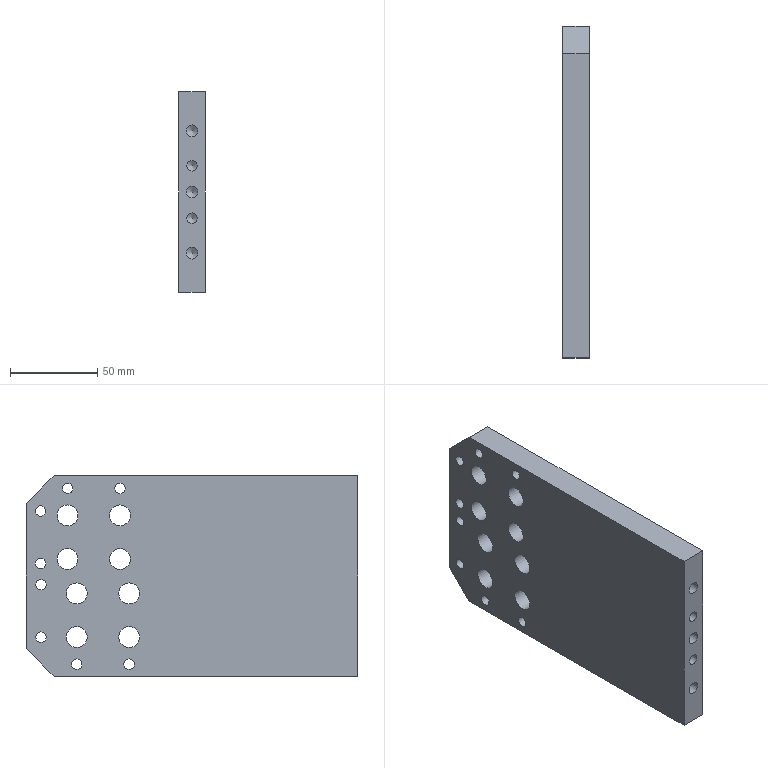Part | NX | features BREP 1 | 1 solid | 38 faces | box 15 x 190 x 115 mm | volume 303398 mm3 | cylinder 23 | plane 8 | cone 7 | commonest cylinder face diameters 6 x10 12 x8 6.8 x3 5 x2
STEP:
#1=CARTESIAN_POINT('',(-7.5,-95.,-57.5));
#2=VERTEX_POINT('',#1);
#3=CARTESIAN_POINT('',(-7.5,79.,-57.5));
#4=VERTEX_POINT('',#3);
#5=CARTESIAN_POINT('',(-7.5,-95.,-57.5));
#6=DIRECTION('',(0.,1.,0.));
#7=VECTOR('',#6,1000.);
#8=LINE('',#5,#7);
#9=EDGE_CURVE('',#2,#4,#8,.T.);
#10=ORIENTED_EDGE('',*,*,#9,.T.);
#11=CARTESIAN_POINT('',(7.5,79.,-57.5));
#12=VERTEX_POINT('',#11);
#13=CARTESIAN_POINT('',(7.5,79.,-57.5));
#14=DIRECTION('',(1.,0.,0.));
#15=VECTOR('',#14,1000.);
#16=LINE('',#13,#15);
#17=EDGE_CURVE('',#4,#12,#16,.T.);
#18=ORIENTED_EDGE('',*,*,#17,.T.);
#19=CARTESIAN_POINT('',(7.5,-95.,-57.5));
#20=VERTEX_POINT('',#19);
#21=CARTESIAN_POINT('',(7.5,-95.,-57.5));
#22=DIRECTION('',(0.,1.,0.));
#23=VECTOR('',#22,1000.);
#24=LINE('',#21,#23);
#25=EDGE_CURVE('',#20,#12,#24,.T.);
#26=ORIENTED_EDGE('',*,*,#25,.F.);
#27=CARTESIAN_POINT('',(7.5,-95.,-57.5));
#28=DIRECTION('',(-1.,0.,0.));
#29=VECTOR('',#28,1000.);
#30=LINE('',#27,#29);
#31=EDGE_CURVE('',#20,#2,#30,.T.);
#32=ORIENTED_EDGE('',*,*,#31,.T.);
#33=EDGE_LOOP('',(#10,#18,#26,#32));
#34=FACE_BOUND('',#33,.T.);
#35=CARTESIAN_POINT('',(7.5,-95.,-57.5));
#36=DIRECTION('',(0.,0.,1.));
#37=DIRECTION('',(-1.,0.,0.));
#38=AXIS2_PLACEMENT_3D('',#35,#36,#37);
#39=PLANE('',#38);
#40=ADVANCED_FACE('',(#34),#39,.F.);
#41=CARTESIAN_POINT('',(0.,95.,-14.5));
#42=VERTEX_POINT('',#41);
#43=CARTESIAN_POINT('',(0.,95.,-17.));
#44=DIRECTION('',(0.,1.,0.));
#45=DIRECTION('',(0.,0.,1.));
#46=AXIS2_PLACEMENT_3D('',#43,#44,#45);
#47=CIRCLE('',#46,2.5);
#48=EDGE_CURVE('',#42,#42,#47,.T.);
#49=ORIENTED_EDGE('',*,*,#48,.F.);
#50=EDGE_LOOP('',(#49));
#51=FACE_BOUND('',#50,.T.);
#52=CARTESIAN_POINT('',(0.,95.,25.5));
#53=VERTEX_POINT('',#52);
#54=CARTESIAN_POINT('',(0.,95.,23.));
#55=DIRECTION('',(0.,1.,0.));
#56=DIRECTION('',(0.,0.,1.));
#57=AXIS2_PLACEMENT_3D('',#54,#55,#56);
#58=CIRCLE('',#57,2.5);
#59=EDGE_CURVE('',#53,#53,#58,.T.);
#60=ORIENTED_EDGE('',*,*,#59,.F.);
#61=EDGE_LOOP('',(#60));
#62=FACE_BOUND('',#61,.T.);
#63=CARTESIAN_POINT('',(-7.5,95.,-41.5));
#64=VERTEX_POINT('',#63);
#65=CARTESIAN_POINT('',(-7.5,95.,41.5));
#66=VERTEX_POINT('',#65);
#67=CARTESIAN_POINT('',(-7.5,95.,57.5));
#68=DIRECTION('',(0.,0.,1.));
#69=VECTOR('',#68,1000.);
#70=LINE('',#67,#69);
#71=EDGE_CURVE('',#64,#66,#70,.T.);
#72=ORIENTED_EDGE('',*,*,#71,.T.);
#73=CARTESIAN_POINT('',(7.5,95.,41.5));
#74=VERTEX_POINT('',#73);
#75=CARTESIAN_POINT('',(7.5,95.,41.5));
#76=DIRECTION('',(1.,0.,0.));
#77=VECTOR('',#76,1000.);
#78=LINE('',#75,#77);
#79=EDGE_CURVE('',#66,#74,#78,.T.);
#80=ORIENTED_EDGE('',*,*,#79,.T.);
#81=CARTESIAN_POINT('',(7.5,95.,-41.5));
#82=VERTEX_POINT('',#81);
#83=CARTESIAN_POINT('',(7.5,95.,57.5));
#84=DIRECTION('',(0.,0.,1.));
#85=VECTOR('',#84,1000.);
#86=LINE('',#83,#85);
#87=EDGE_CURVE('',#82,#74,#86,.T.);
#88=ORIENTED_EDGE('',*,*,#87,.F.);
#89=CARTESIAN_POINT('',(7.5,95.,-41.5));
#90=DIRECTION('',(-1.,0.,0.));
#91=VECTOR('',#90,1000.);
#92=LINE('',#89,#91);
#93=EDGE_CURVE('',#82,#64,#92,.T.);
#94=ORIENTED_EDGE('',*,*,#93,.T.);
#95=EDGE_LOOP('',(#72,#80,#88,#94));
#96=FACE_BOUND('',#95,.T.);
#97=CARTESIAN_POINT('',(7.5,95.,57.5));
#98=DIRECTION('',(0.,-1.,0.));
#99=DIRECTION('',(0.,0.,1.));
#100=AXIS2_PLACEMENT_3D('',#97,#98,#99);
#101=PLANE('',#100);
#102=ADVANCED_FACE('',(#51,#62,#96),#101,.F.);
#103=CARTESIAN_POINT('',(7.5,79.,57.5));
#104=VERTEX_POINT('',#103);
#105=CARTESIAN_POINT('',(7.5,-95.,57.5));
#106=VERTEX_POINT('',#105);
#107=CARTESIAN_POINT('',(7.5,-95.,57.5));
#108=DIRECTION('',(0.,-1.,0.));
#109=VECTOR('',#108,1000.);
#110=LINE('',#107,#109);
#111=EDGE_CURVE('',#104,#106,#110,.T.);
#112=ORIENTED_EDGE('',*,*,#111,.F.);
#113=CARTESIAN_POINT('',(-7.5,79.,57.5));
#114=VERTEX_POINT('',#113);
#115=CARTESIAN_POINT('',(7.5,79.,57.5));
#116=DIRECTION('',(-1.,0.,0.));
#117=VECTOR('',#116,1000.);
#118=LINE('',#115,#117);
#119=EDGE_CURVE('',#104,#114,#118,.T.);
#120=ORIENTED_EDGE('',*,*,#119,.T.);
#121=CARTESIAN_POINT('',(-7.5,-95.,57.5));
#122=VERTEX_POINT('',#121);
#123=CARTESIAN_POINT('',(-7.5,-95.,57.5));
#124=DIRECTION('',(0.,-1.,0.));
#125=VECTOR('',#124,1000.);
#126=LINE('',#123,#125);
#127=EDGE_CURVE('',#114,#122,#126,.T.);
#128=ORIENTED_EDGE('',*,*,#127,.T.);
#129=CARTESIAN_POINT('',(7.5,-95.,57.5));
#130=DIRECTION('',(-1.,0.,0.));
#131=VECTOR('',#130,1000.);
#132=LINE('',#129,#131);
#133=EDGE_CURVE('',#106,#122,#132,.T.);
#134=ORIENTED_EDGE('',*,*,#133,.F.);
#135=EDGE_LOOP('',(#112,#120,#128,#134));
#136=FACE_BOUND('',#135,.T.);
#137=CARTESIAN_POINT('',(7.5,-95.,57.5));
#138=DIRECTION('',(0.,0.,-1.));
#139=DIRECTION('',(1.,0.,0.));
#140=AXIS2_PLACEMENT_3D('',#137,#138,#139);
#141=PLANE('',#140);
#142=ADVANCED_FACE('',(#136),#141,.F.);
#143=CARTESIAN_POINT('',(0.,-95.,-18.));
#144=VERTEX_POINT('',#143);
#145=CARTESIAN_POINT('',(0.,-95.,-15.));
#146=DIRECTION('',(0.,-1.,0.));
#147=DIRECTION('',(0.,0.,-1.));
#148=AXIS2_PLACEMENT_3D('',#145,#146,#147);
#149=CIRCLE('',#148,3.);
#150=EDGE_CURVE('',#144,#144,#149,.T.);
#151=ORIENTED_EDGE('',*,*,#150,.F.);
#152=EDGE_LOOP('',(#151));
#153=FACE_BOUND('',#152,.T.);
#154=CARTESIAN_POINT('',(0.,-95.,12.));
#155=VERTEX_POINT('',#154);
#156=CARTESIAN_POINT('',(0.,-95.,15.));
#157=DIRECTION('',(0.,-1.,0.));
#158=DIRECTION('',(0.,0.,-1.));
#159=AXIS2_PLACEMENT_3D('',#156,#157,#158);
#160=CIRCLE('',#159,3.);
#161=EDGE_CURVE('',#155,#155,#160,.T.);
#162=ORIENTED_EDGE('',*,*,#161,.F.);
#163=EDGE_LOOP('',(#162));
#164=FACE_BOUND('',#163,.T.);
#165=CARTESIAN_POINT('',(0.,-95.,31.6));
#166=VERTEX_POINT('',#165);
#167=CARTESIAN_POINT('',(0.,-95.,35.));
#168=DIRECTION('',(0.,-1.,0.));
#169=DIRECTION('',(0.,0.,-1.));
#170=AXIS2_PLACEMENT_3D('',#167,#168,#169);
#171=CIRCLE('',#170,3.4);
#172=EDGE_CURVE('',#166,#166,#171,.T.);
#173=ORIENTED_EDGE('',*,*,#172,.F.);
#174=EDGE_LOOP('',(#173));
#175=FACE_BOUND('',#174,.T.);
#176=CARTESIAN_POINT('',(0.,-95.,-38.4));
#177=VERTEX_POINT('',#176);
#178=CARTESIAN_POINT('',(0.,-95.,-35.));
#179=DIRECTION('',(0.,-1.,0.));
#180=DIRECTION('',(0.,0.,-1.));
#181=AXIS2_PLACEMENT_3D('',#178,#179,#180);
#182=CIRCLE('',#181,3.4);
#183=EDGE_CURVE('',#177,#177,#182,.T.);
#184=ORIENTED_EDGE('',*,*,#183,.F.);
#185=EDGE_LOOP('',(#184));
#186=FACE_BOUND('',#185,.T.);
#187=CARTESIAN_POINT('',(0.,-95.,-3.4));
#188=VERTEX_POINT('',#187);
#189=CARTESIAN_POINT('',(0.,-95.,0.));
#190=DIRECTION('',(0.,-1.,0.));
#191=DIRECTION('',(0.,0.,-1.));
#192=AXIS2_PLACEMENT_3D('',#189,#190,#191);
#193=CIRCLE('',#192,3.4);
#194=EDGE_CURVE('',#188,#188,#193,.T.);
#195=ORIENTED_EDGE('',*,*,#194,.F.);
#196=EDGE_LOOP('',(#195));
#197=FACE_BOUND('',#196,.T.);
#198=CARTESIAN_POINT('',(-7.5,-95.,57.5));
#199=DIRECTION('',(0.,0.,-1.));
#200=VECTOR('',#199,1000.);
#201=LINE('',#198,#200);
#202=EDGE_CURVE('',#122,#2,#201,.T.);
#203=ORIENTED_EDGE('',*,*,#202,.T.);
#204=ORIENTED_EDGE('',*,*,#31,.F.);
#205=CARTESIAN_POINT('',(7.5,-95.,57.5));
#206=DIRECTION('',(0.,0.,-1.));
#207=VECTOR('',#206,1000.);
#208=LINE('',#205,#207);
#209=EDGE_CURVE('',#106,#20,#208,.T.);
#210=ORIENTED_EDGE('',*,*,#209,.F.);
#211=ORIENTED_EDGE('',*,*,#133,.T.);
#212=EDGE_LOOP('',(#203,#204,#210,#211));
#213=FACE_BOUND('',#212,.T.);
#214=CARTESIAN_POINT('',(7.5,-95.,57.5));
#215=DIRECTION('',(0.,1.,0.));
#216=DIRECTION('',(0.,0.,-1.));
#217=AXIS2_PLACEMENT_3D('',#214,#215,#216);
#218=PLANE('',#217);
#219=ADVANCED_FACE('',(#153,#164,#175,#186,#197,#213),#218,.F.);
#220=CARTESIAN_POINT('',(7.5,66.,-53.5));
#221=VERTEX_POINT('',#220);
#222=CARTESIAN_POINT('',(7.5,66.,-50.5));
#223=DIRECTION('',(1.,0.,0.));
#224=DIRECTION('',(0.,0.,-1.));
#225=AXIS2_PLACEMENT_3D('',#222,#223,#224);
#226=CIRCLE('',#225,3.);
#227=EDGE_CURVE('',#221,#221,#226,.T.);
#228=ORIENTED_EDGE('',*,*,#227,.F.);
#229=EDGE_LOOP('',(#228));
#230=FACE_BOUND('',#229,.T.);
#231=CARTESIAN_POINT('',(7.5,36.,-53.5));
#232=VERTEX_POINT('',#231);
#233=CARTESIAN_POINT('',(7.5,36.,-50.5));
#234=DIRECTION('',(1.,0.,0.));
#235=DIRECTION('',(0.,0.,-1.));
#236=AXIS2_PLACEMENT_3D('',#233,#234,#235);
#237=CIRCLE('',#236,3.);
#238=EDGE_CURVE('',#232,#232,#237,.T.);
#239=ORIENTED_EDGE('',*,*,#238,.F.);
#240=EDGE_LOOP('',(#239));
#241=FACE_BOUND('',#240,.T.);
#242=CARTESIAN_POINT('',(7.5,86.5,-38.));
#243=VERTEX_POINT('',#242);
#244=CARTESIAN_POINT('',(7.5,86.5,-35.));
#245=DIRECTION('',(1.,0.,0.));
#246=DIRECTION('',(0.,0.,-1.));
#247=AXIS2_PLACEMENT_3D('',#244,#245,#246);
#248=CIRCLE('',#247,3.);
#249=EDGE_CURVE('',#243,#243,#248,.T.);
#250=ORIENTED_EDGE('',*,*,#249,.F.);
#251=EDGE_LOOP('',(#250));
#252=FACE_BOUND('',#251,.T.);
#253=CARTESIAN_POINT('',(7.5,86.5,-8.));
#254=VERTEX_POINT('',#253);
#255=CARTESIAN_POINT('',(7.5,86.5,-5.));
#256=DIRECTION('',(1.,0.,0.));
#257=DIRECTION('',(0.,0.,-1.));
#258=AXIS2_PLACEMENT_3D('',#255,#256,#257);
#259=CIRCLE('',#258,3.);
#260=EDGE_CURVE('',#254,#254,#259,.T.);
#261=ORIENTED_EDGE('',*,*,#260,.F.);
#262=EDGE_LOOP('',(#261));
#263=FACE_BOUND('',#262,.T.);
#264=CARTESIAN_POINT('',(7.5,86.759,4.207));
#265=VERTEX_POINT('',#264);
#266=CARTESIAN_POINT('',(7.5,86.759,7.207));
#267=DIRECTION('',(1.,0.,0.));
#268=DIRECTION('',(0.,0.,-1.));
#269=AXIS2_PLACEMENT_3D('',#266,#267,#268);
#270=CIRCLE('',#269,3.);
#271=EDGE_CURVE('',#265,#265,#270,.T.);
#272=ORIENTED_EDGE('',*,*,#271,.F.);
#273=EDGE_LOOP('',(#272));
#274=FACE_BOUND('',#273,.T.);
#275=CARTESIAN_POINT('',(7.5,86.759,34.207));
#276=VERTEX_POINT('',#275);
#277=CARTESIAN_POINT('',(7.5,86.759,37.207));
#278=DIRECTION('',(1.,0.,0.));
#279=DIRECTION('',(0.,0.,-1.));
#280=AXIS2_PLACEMENT_3D('',#277,#278,#279);
#281=CIRCLE('',#280,3.);
#282=EDGE_CURVE('',#276,#276,#281,.T.);
#283=ORIENTED_EDGE('',*,*,#282,.F.);
#284=EDGE_LOOP('',(#283));
#285=FACE_BOUND('',#284,.T.);
#286=CARTESIAN_POINT('',(7.5,71.259,47.207));
#287=VERTEX_POINT('',#286);
#288=CARTESIAN_POINT('',(7.5,71.259,50.207));
#289=DIRECTION('',(1.,0.,0.));
#290=DIRECTION('',(0.,0.,-1.));
#291=AXIS2_PLACEMENT_3D('',#288,#289,#290);
#292=CIRCLE('',#291,3.);
#293=EDGE_CURVE('',#287,#287,#292,.T.);
#294=ORIENTED_EDGE('',*,*,#293,.F.);
#295=EDGE_LOOP('',(#294));
#296=FACE_BOUND('',#295,.T.);
#297=CARTESIAN_POINT('',(7.5,41.259,47.207));
#298=VERTEX_POINT('',#297);
#299=CARTESIAN_POINT('',(7.5,41.259,50.207));
#300=DIRECTION('',(1.,0.,0.));
#301=DIRECTION('',(0.,0.,-1.));
#302=AXIS2_PLACEMENT_3D('',#299,#300,#301);
#303=CIRCLE('',#302,3.);
#304=EDGE_CURVE('',#298,#298,#303,.T.);
#305=ORIENTED_EDGE('',*,*,#304,.F.);
#306=EDGE_LOOP('',(#305));
#307=FACE_BOUND('',#306,.T.);
#308=CARTESIAN_POINT('',(7.5,36.,-29.));
#309=VERTEX_POINT('',#308);
#310=CARTESIAN_POINT('',(7.5,36.,-35.));
#311=DIRECTION('',(-1.,0.,0.));
#312=DIRECTION('',(0.,0.,1.));
#313=AXIS2_PLACEMENT_3D('',#310,#311,#312);
#314=CIRCLE('',#313,6.);
#315=EDGE_CURVE('',#309,#309,#314,.T.);
#316=ORIENTED_EDGE('',*,*,#315,.T.);
#317=EDGE_LOOP('',(#316));
#318=FACE_BOUND('',#317,.T.);
#319=CARTESIAN_POINT('',(7.5,36.,-4.));
#320=VERTEX_POINT('',#319);
#321=CARTESIAN_POINT('',(7.5,36.,-10.));
#322=DIRECTION('',(-1.,0.,0.));
#323=DIRECTION('',(0.,0.,1.));
#324=AXIS2_PLACEMENT_3D('',#321,#322,#323);
#325=CIRCLE('',#324,6.);
#326=EDGE_CURVE('',#320,#320,#325,.T.);
#327=ORIENTED_EDGE('',*,*,#326,.T.);
#328=EDGE_LOOP('',(#327));
#329=FACE_BOUND('',#328,.T.);
#330=CARTESIAN_POINT('',(7.5,66.,-29.));
#331=VERTEX_POINT('',#330);
#332=CARTESIAN_POINT('',(7.5,66.,-35.));
#333=DIRECTION('',(-1.,0.,0.));
#334=DIRECTION('',(0.,0.,1.));
#335=AXIS2_PLACEMENT_3D('',#332,#333,#334);
#336=CIRCLE('',#335,6.);
#337=EDGE_CURVE('',#331,#331,#336,.T.);
#338=ORIENTED_EDGE('',*,*,#337,.T.);
#339=EDGE_LOOP('',(#338));
#340=FACE_BOUND('',#339,.T.);
#341=CARTESIAN_POINT('',(7.5,66.,-4.));
#342=VERTEX_POINT('',#341);
#343=CARTESIAN_POINT('',(7.5,66.,-10.));
#344=DIRECTION('',(-1.,0.,0.));
#345=DIRECTION('',(0.,0.,1.));
#346=AXIS2_PLACEMENT_3D('',#343,#344,#345);
#347=CIRCLE('',#346,6.);
#348=EDGE_CURVE('',#342,#342,#347,.T.);
#349=ORIENTED_EDGE('',*,*,#348,.T.);
#350=EDGE_LOOP('',(#349));
#351=FACE_BOUND('',#350,.T.);
#352=CARTESIAN_POINT('',(7.5,41.259,15.707));
#353=VERTEX_POINT('',#352);
#354=CARTESIAN_POINT('',(7.5,41.259,9.707));
#355=DIRECTION('',(-1.,0.,0.));
#356=DIRECTION('',(0.,0.,1.));
#357=AXIS2_PLACEMENT_3D('',#354,#355,#356);
#358=CIRCLE('',#357,6.);
#359=EDGE_CURVE('',#353,#353,#358,.T.);
#360=ORIENTED_EDGE('',*,*,#359,.T.);
#361=EDGE_LOOP('',(#360));
#362=FACE_BOUND('',#361,.T.);
#363=CARTESIAN_POINT('',(7.5,41.259,40.707));
#364=VERTEX_POINT('',#363);
#365=CARTESIAN_POINT('',(7.5,41.259,34.707));
#366=DIRECTION('',(-1.,0.,0.));
#367=DIRECTION('',(0.,0.,1.));
#368=AXIS2_PLACEMENT_3D('',#365,#366,#367);
#369=CIRCLE('',#368,6.);
#370=EDGE_CURVE('',#364,#364,#369,.T.);
#371=ORIENTED_EDGE('',*,*,#370,.T.);
#372=EDGE_LOOP('',(#371));
#373=FACE_BOUND('',#372,.T.);
#374=CARTESIAN_POINT('',(7.5,71.259,40.707));
#375=VERTEX_POINT('',#374);
#376=CARTESIAN_POINT('',(7.5,71.259,34.707));
#377=DIRECTION('',(-1.,0.,0.));
#378=DIRECTION('',(0.,0.,1.));
#379=AXIS2_PLACEMENT_3D('',#376,#377,#378);
#380=CIRCLE('',#379,6.);
#381=EDGE_CURVE('',#375,#375,#380,.T.);
#382=ORIENTED_EDGE('',*,*,#381,.T.);
#383=EDGE_LOOP('',(#382));
#384=FACE_BOUND('',#383,.T.);
#385=CARTESIAN_POINT('',(7.5,71.259,15.707));
#386=VERTEX_POINT('',#385);
#387=CARTESIAN_POINT('',(7.5,71.259,9.707));
#388=DIRECTION('',(-1.,0.,0.));
#389=DIRECTION('',(0.,0.,1.));
#390=AXIS2_PLACEMENT_3D('',#387,#388,#389);
#391=CIRCLE('',#390,6.);
#392=EDGE_CURVE('',#386,#386,#391,.T.);
#393=ORIENTED_EDGE('',*,*,#392,.T.);
#394=EDGE_LOOP('',(#393));
#395=FACE_BOUND('',#394,.T.);
#396=ORIENTED_EDGE('',*,*,#87,.T.);
#397=CARTESIAN_POINT('',(7.5,79.,57.5));
#398=DIRECTION('',(0.,-0.7071,0.7071));
#399=VECTOR('',#398,1000.);
#400=LINE('',#397,#399);
#401=EDGE_CURVE('',#74,#104,#400,.T.);
#402=ORIENTED_EDGE('',*,*,#401,.T.);
#403=ORIENTED_EDGE('',*,*,#111,.T.);
#404=ORIENTED_EDGE('',*,*,#209,.T.);
#405=ORIENTED_EDGE('',*,*,#25,.T.);
#406=CARTESIAN_POINT('',(7.5,95.,-41.5));
#407=DIRECTION('',(0.,0.7071,0.7071));
#408=VECTOR('',#407,1000.);
#409=LINE('',#406,#408);
#410=EDGE_CURVE('',#12,#82,#409,.T.);
#411=ORIENTED_EDGE('',*,*,#410,.T.);
#412=EDGE_LOOP('',(#396,#402,#403,#404,#405,#411));
#413=FACE_BOUND('',#412,.T.);
#414=CARTESIAN_POINT('',(7.5,0.,0.));
#415=DIRECTION('',(-1.,0.,0.));
#416=DIRECTION('',(0.,0.,-1.));
#417=AXIS2_PLACEMENT_3D('',#414,#415,#416);
#418=PLANE('',#417);
#419=ADVANCED_FACE('',(#230,#241,#252,#263,#274,#285,#296,#307,#318,#329,#340,#351,#362,#373,#384,#395,#413),#418,.F.);
#420=CARTESIAN_POINT('',(-7.5,66.,-53.5));
#421=VERTEX_POINT('',#420);
#422=CARTESIAN_POINT('',(-7.5,66.,-50.5));
#423=DIRECTION('',(1.,0.,0.));
#424=DIRECTION('',(0.,0.,-1.));
#425=AXIS2_PLACEMENT_3D('',#422,#423,#424);
#426=CIRCLE('',#425,3.);
#427=EDGE_CURVE('',#421,#421,#426,.T.);
#428=ORIENTED_EDGE('',*,*,#427,.T.);
#429=EDGE_LOOP('',(#428));
#430=FACE_BOUND('',#429,.T.);
#431=CARTESIAN_POINT('',(-7.5,36.,-53.5));
#432=VERTEX_POINT('',#431);
#433=CARTESIAN_POINT('',(-7.5,36.,-50.5));
#434=DIRECTION('',(1.,0.,0.));
#435=DIRECTION('',(0.,0.,-1.));
#436=AXIS2_PLACEMENT_3D('',#433,#434,#435);
#437=CIRCLE('',#436,3.);
#438=EDGE_CURVE('',#432,#432,#437,.T.);
#439=ORIENTED_EDGE('',*,*,#438,.T.);
#440=EDGE_LOOP('',(#439));
#441=FACE_BOUND('',#440,.T.);
#442=CARTESIAN_POINT('',(-7.5,86.5,-38.));
#443=VERTEX_POINT('',#442);
#444=CARTESIAN_POINT('',(-7.5,86.5,-35.));
#445=DIRECTION('',(1.,0.,0.));
#446=DIRECTION('',(0.,0.,-1.));
#447=AXIS2_PLACEMENT_3D('',#444,#445,#446);
#448=CIRCLE('',#447,3.);
#449=EDGE_CURVE('',#443,#443,#448,.T.);
#450=ORIENTED_EDGE('',*,*,#449,.T.);
#451=EDGE_LOOP('',(#450));
#452=FACE_BOUND('',#451,.T.);
#453=CARTESIAN_POINT('',(-7.5,86.5,-8.));
#454=VERTEX_POINT('',#453);
#455=CARTESIAN_POINT('',(-7.5,86.5,-5.));
#456=DIRECTION('',(1.,0.,0.));
#457=DIRECTION('',(0.,0.,-1.));
#458=AXIS2_PLACEMENT_3D('',#455,#456,#457);
#459=CIRCLE('',#458,3.);
#460=EDGE_CURVE('',#454,#454,#459,.T.);
#461=ORIENTED_EDGE('',*,*,#460,.T.);
#462=EDGE_LOOP('',(#461));
#463=FACE_BOUND('',#462,.T.);
#464=CARTESIAN_POINT('',(-7.5,86.759,4.207));
#465=VERTEX_POINT('',#464);
#466=CARTESIAN_POINT('',(-7.5,86.759,7.207));
#467=DIRECTION('',(1.,0.,0.));
#468=DIRECTION('',(0.,0.,-1.));
#469=AXIS2_PLACEMENT_3D('',#466,#467,#468);
#470=CIRCLE('',#469,3.);
#471=EDGE_CURVE('',#465,#465,#470,.T.);
#472=ORIENTED_EDGE('',*,*,#471,.T.);
#473=EDGE_LOOP('',(#472));
#474=FACE_BOUND('',#473,.T.);
#475=CARTESIAN_POINT('',(-7.5,86.759,34.207));
#476=VERTEX_POINT('',#475);
#477=CARTESIAN_POINT('',(-7.5,86.759,37.207));
#478=DIRECTION('',(1.,0.,0.));
#479=DIRECTION('',(0.,0.,-1.));
#480=AXIS2_PLACEMENT_3D('',#477,#478,#479);
#481=CIRCLE('',#480,3.);
#482=EDGE_CURVE('',#476,#476,#481,.T.);
#483=ORIENTED_EDGE('',*,*,#482,.T.);
#484=EDGE_LOOP('',(#483));
#485=FACE_BOUND('',#484,.T.);
#486=CARTESIAN_POINT('',(-7.5,71.259,47.207));
#487=VERTEX_POINT('',#486);
#488=CARTESIAN_POINT('',(-7.5,71.259,50.207));
#489=DIRECTION('',(1.,0.,0.));
#490=DIRECTION('',(0.,0.,-1.));
#491=AXIS2_PLACEMENT_3D('',#488,#489,#490);
#492=CIRCLE('',#491,3.);
#493=EDGE_CURVE('',#487,#487,#492,.T.);
#494=ORIENTED_EDGE('',*,*,#493,.T.);
#495=EDGE_LOOP('',(#494));
#496=FACE_BOUND('',#495,.T.);
#497=CARTESIAN_POINT('',(-7.5,41.259,47.207));
#498=VERTEX_POINT('',#497);
#499=CARTESIAN_POINT('',(-7.5,41.259,50.207));
#500=DIRECTION('',(1.,0.,0.));
#501=DIRECTION('',(0.,0.,-1.));
#502=AXIS2_PLACEMENT_3D('',#499,#500,#501);
#503=CIRCLE('',#502,3.);
#504=EDGE_CURVE('',#498,#498,#503,.T.);
#505=ORIENTED_EDGE('',*,*,#504,.T.);
#506=EDGE_LOOP('',(#505));
#507=FACE_BOUND('',#506,.T.);
#508=CARTESIAN_POINT('',(-7.5,36.,-29.));
#509=VERTEX_POINT('',#508);
#510=CARTESIAN_POINT('',(-7.5,36.,-35.));
#511=DIRECTION('',(-1.,0.,0.));
#512=DIRECTION('',(0.,0.,1.));
#513=AXIS2_PLACEMENT_3D('',#510,#511,#512);
#514=CIRCLE('',#513,6.);
#515=EDGE_CURVE('',#509,#509,#514,.T.);
#516=ORIENTED_EDGE('',*,*,#515,.F.);
#517=EDGE_LOOP('',(#516));
#518=FACE_BOUND('',#517,.T.);
#519=CARTESIAN_POINT('',(-7.5,36.,-4.));
#520=VERTEX_POINT('',#519);
#521=CARTESIAN_POINT('',(-7.5,36.,-10.));
#522=DIRECTION('',(-1.,0.,0.));
#523=DIRECTION('',(0.,0.,1.));
#524=AXIS2_PLACEMENT_3D('',#521,#522,#523);
#525=CIRCLE('',#524,6.);
#526=EDGE_CURVE('',#520,#520,#525,.T.);
#527=ORIENTED_EDGE('',*,*,#526,.F.);
#528=EDGE_LOOP('',(#527));
#529=FACE_BOUND('',#528,.T.);
#530=CARTESIAN_POINT('',(-7.5,66.,-29.));
#531=VERTEX_POINT('',#530);
#532=CARTESIAN_POINT('',(-7.5,66.,-35.));
#533=DIRECTION('',(-1.,0.,0.));
#534=DIRECTION('',(0.,0.,1.));
#535=AXIS2_PLACEMENT_3D('',#532,#533,#534);
#536=CIRCLE('',#535,6.);
#537=EDGE_CURVE('',#531,#531,#536,.T.);
#538=ORIENTED_EDGE('',*,*,#537,.F.);
#539=EDGE_LOOP('',(#538));
#540=FACE_BOUND('',#539,.T.);
#541=CARTESIAN_POINT('',(-7.5,66.,-4.));
#542=VERTEX_POINT('',#541);
#543=CARTESIAN_POINT('',(-7.5,66.,-10.));
#544=DIRECTION('',(-1.,0.,0.));
#545=DIRECTION('',(0.,0.,1.));
#546=AXIS2_PLACEMENT_3D('',#543,#544,#545);
#547=CIRCLE('',#546,6.);
#548=EDGE_CURVE('',#542,#542,#547,.T.);
#549=ORIENTED_EDGE('',*,*,#548,.F.);
#550=EDGE_LOOP('',(#549));
#551=FACE_BOUND('',#550,.T.);
#552=CARTESIAN_POINT('',(-7.5,41.259,15.707));
#553=VERTEX_POINT('',#552);
#554=CARTESIAN_POINT('',(-7.5,41.259,9.707));
#555=DIRECTION('',(-1.,0.,0.));
#556=DIRECTION('',(0.,0.,1.));
#557=AXIS2_PLACEMENT_3D('',#554,#555,#556);
#558=CIRCLE('',#557,6.);
#559=EDGE_CURVE('',#553,#553,#558,.T.);
#560=ORIENTED_EDGE('',*,*,#559,.F.);
#561=EDGE_LOOP('',(#560));
#562=FACE_BOUND('',#561,.T.);
#563=CARTESIAN_POINT('',(-7.5,41.259,40.707));
#564=VERTEX_POINT('',#563);
#565=CARTESIAN_POINT('',(-7.5,41.259,34.707));
#566=DIRECTION('',(-1.,0.,0.));
#567=DIRECTION('',(0.,0.,1.));
#568=AXIS2_PLACEMENT_3D('',#565,#566,#567);
#569=CIRCLE('',#568,6.);
#570=EDGE_CURVE('',#564,#564,#569,.T.);
#571=ORIENTED_EDGE('',*,*,#570,.F.);
#572=EDGE_LOOP('',(#571));
#573=FACE_BOUND('',#572,.T.);
#574=CARTESIAN_POINT('',(-7.5,71.259,40.707));
#575=VERTEX_POINT('',#574);
#576=CARTESIAN_POINT('',(-7.5,71.259,34.707));
#577=DIRECTION('',(-1.,0.,0.));
#578=DIRECTION('',(0.,0.,1.));
#579=AXIS2_PLACEMENT_3D('',#576,#577,#578);
#580=CIRCLE('',#579,6.);
#581=EDGE_CURVE('',#575,#575,#580,.T.);
#582=ORIENTED_EDGE('',*,*,#581,.F.);
#583=EDGE_LOOP('',(#582));
#584=FACE_BOUND('',#583,.T.);
#585=CARTESIAN_POINT('',(-7.5,71.259,15.707));
#586=VERTEX_POINT('',#585);
#587=CARTESIAN_POINT('',(-7.5,71.259,9.707));
#588=DIRECTION('',(-1.,0.,0.));
#589=DIRECTION('',(0.,0.,1.));
#590=AXIS2_PLACEMENT_3D('',#587,#588,#589);
#591=CIRCLE('',#590,6.);
#592=EDGE_CURVE('',#586,#586,#591,.T.);
#593=ORIENTED_EDGE('',*,*,#592,.F.);
#594=EDGE_LOOP('',(#593));
#595=FACE_BOUND('',#594,.T.);
#596=ORIENTED_EDGE('',*,*,#127,.F.);
#597=CARTESIAN_POINT('',(-7.5,68.25,68.25));
#598=DIRECTION('',(0.,0.7071,-0.7071));
#599=VECTOR('',#598,1000.);
#600=LINE('',#597,#599);
#601=EDGE_CURVE('',#114,#66,#600,.T.);
#602=ORIENTED_EDGE('',*,*,#601,.T.);
#603=ORIENTED_EDGE('',*,*,#71,.F.);
#604=CARTESIAN_POINT('',(-7.5,68.25,-68.25));
#605=DIRECTION('',(0.,-0.7071,-0.7071));
#606=VECTOR('',#605,1000.);
#607=LINE('',#604,#606);
#608=EDGE_CURVE('',#64,#4,#607,.T.);
#609=ORIENTED_EDGE('',*,*,#608,.T.);
#610=ORIENTED_EDGE('',*,*,#9,.F.);
#611=ORIENTED_EDGE('',*,*,#202,.F.);
#612=EDGE_LOOP('',(#596,#602,#603,#609,#610,#611));
#613=FACE_BOUND('',#612,.T.);
#614=CARTESIAN_POINT('',(-7.5,0.,0.));
#615=DIRECTION('',(-1.,0.,0.));
#616=DIRECTION('',(0.,0.,-1.));
#617=AXIS2_PLACEMENT_3D('',#614,#615,#616);
#618=PLANE('',#617);
#619=ADVANCED_FACE('',(#430,#441,#452,#463,#474,#485,#496,#507,#518,#529,#540,#551,#562,#573,#584,#595,#613),#618,.T.);
#620=ORIENTED_EDGE('',*,*,#392,.F.);
#621=EDGE_LOOP('',(#620));
#622=FACE_BOUND('',#621,.T.);
#623=ORIENTED_EDGE('',*,*,#592,.T.);
#624=EDGE_LOOP('',(#623));
#625=FACE_BOUND('',#624,.T.);
#626=CARTESIAN_POINT('',(-7.5,71.259,9.707));
#627=DIRECTION('',(-1.,0.,0.));
#628=DIRECTION('',(0.,0.,-1.));
#629=AXIS2_PLACEMENT_3D('',#626,#627,#628);
#630=CYLINDRICAL_SURFACE('',#629,6.);
#631=ADVANCED_FACE('',(#622,#625),#630,.F.);
#632=ORIENTED_EDGE('',*,*,#381,.F.);
#633=EDGE_LOOP('',(#632));
#634=FACE_BOUND('',#633,.T.);
#635=ORIENTED_EDGE('',*,*,#581,.T.);
#636=EDGE_LOOP('',(#635));
#637=FACE_BOUND('',#636,.T.);
#638=CARTESIAN_POINT('',(-7.5,71.259,34.707));
#639=DIRECTION('',(-1.,0.,0.));
#640=DIRECTION('',(0.,0.,-1.));
#641=AXIS2_PLACEMENT_3D('',#638,#639,#640);
#642=CYLINDRICAL_SURFACE('',#641,6.);
#643=ADVANCED_FACE('',(#634,#637),#642,.F.);
#644=ORIENTED_EDGE('',*,*,#370,.F.);
#645=EDGE_LOOP('',(#644));
#646=FACE_BOUND('',#645,.T.);
#647=ORIENTED_EDGE('',*,*,#570,.T.);
#648=EDGE_LOOP('',(#647));
#649=FACE_BOUND('',#648,.T.);
#650=CARTESIAN_POINT('',(-7.5,41.259,34.707));
#651=DIRECTION('',(-1.,0.,0.));
#652=DIRECTION('',(0.,0.,-1.));
#653=AXIS2_PLACEMENT_3D('',#650,#651,#652);
#654=CYLINDRICAL_SURFACE('',#653,6.);
#655=ADVANCED_FACE('',(#646,#649),#654,.F.);
#656=ORIENTED_EDGE('',*,*,#359,.F.);
#657=EDGE_LOOP('',(#656));
#658=FACE_BOUND('',#657,.T.);
#659=ORIENTED_EDGE('',*,*,#559,.T.);
#660=EDGE_LOOP('',(#659));
#661=FACE_BOUND('',#660,.T.);
#662=CARTESIAN_POINT('',(-7.5,41.259,9.707));
#663=DIRECTION('',(-1.,0.,0.));
#664=DIRECTION('',(0.,0.,-1.));
#665=AXIS2_PLACEMENT_3D('',#662,#663,#664);
#666=CYLINDRICAL_SURFACE('',#665,6.);
#667=ADVANCED_FACE('',(#658,#661),#666,.F.);
#668=ORIENTED_EDGE('',*,*,#348,.F.);
#669=EDGE_LOOP('',(#668));
#670=FACE_BOUND('',#669,.T.);
#671=ORIENTED_EDGE('',*,*,#548,.T.);
#672=EDGE_LOOP('',(#671));
#673=FACE_BOUND('',#672,.T.);
#674=CARTESIAN_POINT('',(-7.5,66.,-10.));
#675=DIRECTION('',(-1.,0.,0.));
#676=DIRECTION('',(0.,0.,-1.));
#677=AXIS2_PLACEMENT_3D('',#674,#675,#676);
#678=CYLINDRICAL_SURFACE('',#677,6.);
#679=ADVANCED_FACE('',(#670,#673),#678,.F.);
#680=ORIENTED_EDGE('',*,*,#337,.F.);
#681=EDGE_LOOP('',(#680));
#682=FACE_BOUND('',#681,.T.);
#683=ORIENTED_EDGE('',*,*,#537,.T.);
#684=EDGE_LOOP('',(#683));
#685=FACE_BOUND('',#684,.T.);
#686=CARTESIAN_POINT('',(-7.5,66.,-35.));
#687=DIRECTION('',(-1.,0.,0.));
#688=DIRECTION('',(0.,0.,-1.));
#689=AXIS2_PLACEMENT_3D('',#686,#687,#688);
#690=CYLINDRICAL_SURFACE('',#689,6.);
#691=ADVANCED_FACE('',(#682,#685),#690,.F.);
#692=ORIENTED_EDGE('',*,*,#326,.F.);
#693=EDGE_LOOP('',(#692));
#694=FACE_BOUND('',#693,.T.);
#695=ORIENTED_EDGE('',*,*,#526,.T.);
#696=EDGE_LOOP('',(#695));
#697=FACE_BOUND('',#696,.T.);
#698=CARTESIAN_POINT('',(-7.5,36.,-10.));
#699=DIRECTION('',(-1.,0.,0.));
#700=DIRECTION('',(0.,0.,-1.));
#701=AXIS2_PLACEMENT_3D('',#698,#699,#700);
#702=CYLINDRICAL_SURFACE('',#701,6.);
#703=ADVANCED_FACE('',(#694,#697),#702,.F.);
#704=ORIENTED_EDGE('',*,*,#315,.F.);
#705=EDGE_LOOP('',(#704));
#706=FACE_BOUND('',#705,.T.);
#707=ORIENTED_EDGE('',*,*,#515,.T.);
#708=EDGE_LOOP('',(#707));
#709=FACE_BOUND('',#708,.T.);
#710=CARTESIAN_POINT('',(-7.5,36.,-35.));
#711=DIRECTION('',(-1.,0.,0.));
#712=DIRECTION('',(0.,0.,-1.));
#713=AXIS2_PLACEMENT_3D('',#710,#711,#712);
#714=CYLINDRICAL_SURFACE('',#713,6.);
#715=ADVANCED_FACE('',(#706,#709),#714,.F.);
#716=ORIENTED_EDGE('',*,*,#504,.F.);
#717=EDGE_LOOP('',(#716));
#718=FACE_BOUND('',#717,.T.);
#719=ORIENTED_EDGE('',*,*,#304,.T.);
#720=EDGE_LOOP('',(#719));
#721=FACE_BOUND('',#720,.T.);
#722=CARTESIAN_POINT('',(7.5,41.259,50.207));
#723=DIRECTION('',(1.,0.,0.));
#724=DIRECTION('',(0.,0.,1.));
#725=AXIS2_PLACEMENT_3D('',#722,#723,#724);
#726=CYLINDRICAL_SURFACE('',#725,3.);
#727=ADVANCED_FACE('',(#718,#721),#726,.F.);
#728=ORIENTED_EDGE('',*,*,#493,.F.);
#729=EDGE_LOOP('',(#728));
#730=FACE_BOUND('',#729,.T.);
#731=ORIENTED_EDGE('',*,*,#293,.T.);
#732=EDGE_LOOP('',(#731));
#733=FACE_BOUND('',#732,.T.);
#734=CARTESIAN_POINT('',(7.5,71.259,50.207));
#735=DIRECTION('',(1.,0.,0.));
#736=DIRECTION('',(0.,0.,1.));
#737=AXIS2_PLACEMENT_3D('',#734,#735,#736);
#738=CYLINDRICAL_SURFACE('',#737,3.);
#739=ADVANCED_FACE('',(#730,#733),#738,.F.);
#740=ORIENTED_EDGE('',*,*,#482,.F.);
#741=EDGE_LOOP('',(#740));
#742=FACE_BOUND('',#741,.T.);
#743=ORIENTED_EDGE('',*,*,#282,.T.);
#744=EDGE_LOOP('',(#743));
#745=FACE_BOUND('',#744,.T.);
#746=CARTESIAN_POINT('',(7.5,86.759,37.207));
#747=DIRECTION('',(1.,0.,0.));
#748=DIRECTION('',(0.,0.,1.));
#749=AXIS2_PLACEMENT_3D('',#746,#747,#748);
#750=CYLINDRICAL_SURFACE('',#749,3.);
#751=ADVANCED_FACE('',(#742,#745),#750,.F.);
#752=ORIENTED_EDGE('',*,*,#471,.F.);
#753=EDGE_LOOP('',(#752));
#754=FACE_BOUND('',#753,.T.);
#755=ORIENTED_EDGE('',*,*,#271,.T.);
#756=EDGE_LOOP('',(#755));
#757=FACE_BOUND('',#756,.T.);
#758=CARTESIAN_POINT('',(7.5,86.759,7.207));
#759=DIRECTION('',(1.,0.,0.));
#760=DIRECTION('',(0.,0.,1.));
#761=AXIS2_PLACEMENT_3D('',#758,#759,#760);
#762=CYLINDRICAL_SURFACE('',#761,3.);
#763=ADVANCED_FACE('',(#754,#757),#762,.F.);
#764=ORIENTED_EDGE('',*,*,#460,.F.);
#765=EDGE_LOOP('',(#764));
#766=FACE_BOUND('',#765,.T.);
#767=ORIENTED_EDGE('',*,*,#260,.T.);
#768=EDGE_LOOP('',(#767));
#769=FACE_BOUND('',#768,.T.);
#770=CARTESIAN_POINT('',(7.5,86.5,-5.));
#771=DIRECTION('',(1.,0.,0.));
#772=DIRECTION('',(0.,0.,1.));
#773=AXIS2_PLACEMENT_3D('',#770,#771,#772);
#774=CYLINDRICAL_SURFACE('',#773,3.);
#775=ADVANCED_FACE('',(#766,#769),#774,.F.);
#776=ORIENTED_EDGE('',*,*,#449,.F.);
#777=EDGE_LOOP('',(#776));
#778=FACE_BOUND('',#777,.T.);
#779=ORIENTED_EDGE('',*,*,#249,.T.);
#780=EDGE_LOOP('',(#779));
#781=FACE_BOUND('',#780,.T.);
#782=CARTESIAN_POINT('',(7.5,86.5,-35.));
#783=DIRECTION('',(1.,0.,0.));
#784=DIRECTION('',(0.,0.,1.));
#785=AXIS2_PLACEMENT_3D('',#782,#783,#784);
#786=CYLINDRICAL_SURFACE('',#785,3.);
#787=ADVANCED_FACE('',(#778,#781),#786,.F.);
#788=ORIENTED_EDGE('',*,*,#438,.F.);
#789=EDGE_LOOP('',(#788));
#790=FACE_BOUND('',#789,.T.);
#791=ORIENTED_EDGE('',*,*,#238,.T.);
#792=EDGE_LOOP('',(#791));
#793=FACE_BOUND('',#792,.T.);
#794=CARTESIAN_POINT('',(7.5,36.,-50.5));
#795=DIRECTION('',(1.,0.,0.));
#796=DIRECTION('',(0.,0.,1.));
#797=AXIS2_PLACEMENT_3D('',#794,#795,#796);
#798=CYLINDRICAL_SURFACE('',#797,3.);
#799=ADVANCED_FACE('',(#790,#793),#798,.F.);
#800=ORIENTED_EDGE('',*,*,#427,.F.);
#801=EDGE_LOOP('',(#800));
#802=FACE_BOUND('',#801,.T.);
#803=ORIENTED_EDGE('',*,*,#227,.T.);
#804=EDGE_LOOP('',(#803));
#805=FACE_BOUND('',#804,.T.);
#806=CARTESIAN_POINT('',(7.5,66.,-50.5));
#807=DIRECTION('',(1.,0.,0.));
#808=DIRECTION('',(0.,0.,1.));
#809=AXIS2_PLACEMENT_3D('',#806,#807,#808);
#810=CYLINDRICAL_SURFACE('',#809,3.);
#811=ADVANCED_FACE('',(#802,#805),#810,.F.);
#812=CARTESIAN_POINT('',(0.,-73.207,0.));
#813=VERTEX_POINT('',#812);
#814=VERTEX_LOOP('',#813);
#815=FACE_BOUND('',#814,.T.);
#816=CARTESIAN_POINT('',(0.,-75.25,-3.4));
#817=VERTEX_POINT('',#816);
#818=CARTESIAN_POINT('',(0.,-75.25,0.));
#819=DIRECTION('',(0.,-1.,0.));
#820=DIRECTION('',(0.,0.,-1.));
#821=AXIS2_PLACEMENT_3D('',#818,#819,#820);
#822=CIRCLE('',#821,3.4);
#823=EDGE_CURVE('',#817,#817,#822,.T.);
#824=ORIENTED_EDGE('',*,*,#823,.T.);
#825=EDGE_LOOP('',(#824));
#826=FACE_BOUND('',#825,.T.);
#827=CARTESIAN_POINT('',(0.,-75.25,0.));
#828=DIRECTION('',(0.,-1.,0.));
#829=DIRECTION('',(0.,0.,1.));
#830=AXIS2_PLACEMENT_3D('',#827,#828,#829);
#831=CONICAL_SURFACE('',#830,3.4,1.03);
#832=ADVANCED_FACE('',(#815,#826),#831,.F.);
#833=ORIENTED_EDGE('',*,*,#823,.F.);
#834=EDGE_LOOP('',(#833));
#835=FACE_BOUND('',#834,.T.);
#836=ORIENTED_EDGE('',*,*,#194,.T.);
#837=EDGE_LOOP('',(#836));
#838=FACE_BOUND('',#837,.T.);
#839=CARTESIAN_POINT('',(0.,-95.,0.));
#840=DIRECTION('',(0.,-1.,0.));
#841=DIRECTION('',(0.,0.,1.));
#842=AXIS2_PLACEMENT_3D('',#839,#840,#841);
#843=CYLINDRICAL_SURFACE('',#842,3.4);
#844=ADVANCED_FACE('',(#835,#838),#843,.F.);
#845=CARTESIAN_POINT('',(0.,-73.207,-35.));
#846=VERTEX_POINT('',#845);
#847=VERTEX_LOOP('',#846);
#848=FACE_BOUND('',#847,.T.);
#849=CARTESIAN_POINT('',(0.,-75.25,-38.4));
#850=VERTEX_POINT('',#849);
#851=CARTESIAN_POINT('',(0.,-75.25,-35.));
#852=DIRECTION('',(0.,-1.,0.));
#853=DIRECTION('',(0.,0.,-1.));
#854=AXIS2_PLACEMENT_3D('',#851,#852,#853);
#855=CIRCLE('',#854,3.4);
#856=EDGE_CURVE('',#850,#850,#855,.T.);
#857=ORIENTED_EDGE('',*,*,#856,.T.);
#858=EDGE_LOOP('',(#857));
#859=FACE_BOUND('',#858,.T.);
#860=CARTESIAN_POINT('',(0.,-75.25,-35.));
#861=DIRECTION('',(0.,-1.,0.));
#862=DIRECTION('',(0.,0.,1.));
#863=AXIS2_PLACEMENT_3D('',#860,#861,#862);
#864=CONICAL_SURFACE('',#863,3.4,1.03);
#865=ADVANCED_FACE('',(#848,#859),#864,.F.);
#866=ORIENTED_EDGE('',*,*,#856,.F.);
#867=EDGE_LOOP('',(#866));
#868=FACE_BOUND('',#867,.T.);
#869=ORIENTED_EDGE('',*,*,#183,.T.);
#870=EDGE_LOOP('',(#869));
#871=FACE_BOUND('',#870,.T.);
#872=CARTESIAN_POINT('',(0.,-95.,-35.));
#873=DIRECTION('',(0.,-1.,0.));
#874=DIRECTION('',(0.,0.,1.));
#875=AXIS2_PLACEMENT_3D('',#872,#873,#874);
#876=CYLINDRICAL_SURFACE('',#875,3.4);
#877=ADVANCED_FACE('',(#868,#871),#876,.F.);
#878=CARTESIAN_POINT('',(0.,-73.207,35.));
#879=VERTEX_POINT('',#878);
#880=VERTEX_LOOP('',#879);
#881=FACE_BOUND('',#880,.T.);
#882=CARTESIAN_POINT('',(0.,-75.25,31.6));
#883=VERTEX_POINT('',#882);
#884=CARTESIAN_POINT('',(0.,-75.25,35.));
#885=DIRECTION('',(0.,-1.,0.));
#886=DIRECTION('',(0.,0.,-1.));
#887=AXIS2_PLACEMENT_3D('',#884,#885,#886);
#888=CIRCLE('',#887,3.4);
#889=EDGE_CURVE('',#883,#883,#888,.T.);
#890=ORIENTED_EDGE('',*,*,#889,.T.);
#891=EDGE_LOOP('',(#890));
#892=FACE_BOUND('',#891,.T.);
#893=CARTESIAN_POINT('',(0.,-75.25,35.));
#894=DIRECTION('',(0.,-1.,0.));
#895=DIRECTION('',(0.,0.,1.));
#896=AXIS2_PLACEMENT_3D('',#893,#894,#895);
#897=CONICAL_SURFACE('',#896,3.4,1.03);
#898=ADVANCED_FACE('',(#881,#892),#897,.F.);
#899=ORIENTED_EDGE('',*,*,#889,.F.);
#900=EDGE_LOOP('',(#899));
#901=FACE_BOUND('',#900,.T.);
#902=ORIENTED_EDGE('',*,*,#172,.T.);
#903=EDGE_LOOP('',(#902));
#904=FACE_BOUND('',#903,.T.);
#905=CARTESIAN_POINT('',(0.,-95.,35.));
#906=DIRECTION('',(0.,-1.,0.));
#907=DIRECTION('',(0.,0.,1.));
#908=AXIS2_PLACEMENT_3D('',#905,#906,#907);
#909=CYLINDRICAL_SURFACE('',#908,3.4);
#910=ADVANCED_FACE('',(#901,#904),#909,.F.);
#911=CARTESIAN_POINT('',(0.,-81.197,15.));
#912=VERTEX_POINT('',#911);
#913=VERTEX_LOOP('',#912);
#914=FACE_BOUND('',#913,.T.);
#915=CARTESIAN_POINT('',(0.,-83.,12.));
#916=VERTEX_POINT('',#915);
#917=CARTESIAN_POINT('',(0.,-83.,15.));
#918=DIRECTION('',(0.,-1.,0.));
#919=DIRECTION('',(0.,0.,-1.));
#920=AXIS2_PLACEMENT_3D('',#917,#918,#919);
#921=CIRCLE('',#920,3.);
#922=EDGE_CURVE('',#916,#916,#921,.T.);
#923=ORIENTED_EDGE('',*,*,#922,.T.);
#924=EDGE_LOOP('',(#923));
#925=FACE_BOUND('',#924,.T.);
#926=CARTESIAN_POINT('',(0.,-83.,15.));
#927=DIRECTION('',(0.,-1.,0.));
#928=DIRECTION('',(0.,0.,1.));
#929=AXIS2_PLACEMENT_3D('',#926,#927,#928);
#930=CONICAL_SURFACE('',#929,3.,1.03);
#931=ADVANCED_FACE('',(#914,#925),#930,.F.);
#932=ORIENTED_EDGE('',*,*,#922,.F.);
#933=EDGE_LOOP('',(#932));
#934=FACE_BOUND('',#933,.T.);
#935=ORIENTED_EDGE('',*,*,#161,.T.);
#936=EDGE_LOOP('',(#935));
#937=FACE_BOUND('',#936,.T.);
#938=CARTESIAN_POINT('',(0.,-95.,15.));
#939=DIRECTION('',(0.,-1.,0.));
#940=DIRECTION('',(0.,0.,1.));
#941=AXIS2_PLACEMENT_3D('',#938,#939,#940);
#942=CYLINDRICAL_SURFACE('',#941,3.);
#943=ADVANCED_FACE('',(#934,#937),#942,.F.);
#944=CARTESIAN_POINT('',(0.,-81.197,-15.));
#945=VERTEX_POINT('',#944);
#946=VERTEX_LOOP('',#945);
#947=FACE_BOUND('',#946,.T.);
#948=CARTESIAN_POINT('',(0.,-83.,-18.));
#949=VERTEX_POINT('',#948);
#950=CARTESIAN_POINT('',(0.,-83.,-15.));
#951=DIRECTION('',(0.,-1.,0.));
#952=DIRECTION('',(0.,0.,-1.));
#953=AXIS2_PLACEMENT_3D('',#950,#951,#952);
#954=CIRCLE('',#953,3.);
#955=EDGE_CURVE('',#949,#949,#954,.T.);
#956=ORIENTED_EDGE('',*,*,#955,.T.);
#957=EDGE_LOOP('',(#956));
#958=FACE_BOUND('',#957,.T.);
#959=CARTESIAN_POINT('',(0.,-83.,-15.));
#960=DIRECTION('',(0.,-1.,0.));
#961=DIRECTION('',(0.,0.,1.));
#962=AXIS2_PLACEMENT_3D('',#959,#960,#961);
#963=CONICAL_SURFACE('',#962,3.,1.03);
#964=ADVANCED_FACE('',(#947,#958),#963,.F.);
#965=ORIENTED_EDGE('',*,*,#955,.F.);
#966=EDGE_LOOP('',(#965));
#967=FACE_BOUND('',#966,.T.);
#968=ORIENTED_EDGE('',*,*,#150,.T.);
#969=EDGE_LOOP('',(#968));
#970=FACE_BOUND('',#969,.T.);
#971=CARTESIAN_POINT('',(0.,-95.,-15.));
#972=DIRECTION('',(0.,-1.,0.));
#973=DIRECTION('',(0.,0.,1.));
#974=AXIS2_PLACEMENT_3D('',#971,#972,#973);
#975=CYLINDRICAL_SURFACE('',#974,3.);
#976=ADVANCED_FACE('',(#967,#970),#975,.F.);
#977=ORIENTED_EDGE('',*,*,#401,.F.);
#978=ORIENTED_EDGE('',*,*,#79,.F.);
#979=ORIENTED_EDGE('',*,*,#601,.F.);
#980=ORIENTED_EDGE('',*,*,#119,.F.);
#981=EDGE_LOOP('',(#977,#978,#979,#980));
#982=FACE_BOUND('',#981,.T.);
#983=CARTESIAN_POINT('',(7.5,79.,57.5));
#984=DIRECTION('',(0.,-0.7071,-0.7071));
#985=DIRECTION('',(1.,0.,0.));
#986=AXIS2_PLACEMENT_3D('',#983,#984,#985);
#987=PLANE('',#986);
#988=ADVANCED_FACE('',(#982),#987,.F.);
#989=ORIENTED_EDGE('',*,*,#410,.F.);
#990=ORIENTED_EDGE('',*,*,#17,.F.);
#991=ORIENTED_EDGE('',*,*,#608,.F.);
#992=ORIENTED_EDGE('',*,*,#93,.F.);
#993=EDGE_LOOP('',(#989,#990,#991,#992));
#994=FACE_BOUND('',#993,.T.);
#995=CARTESIAN_POINT('',(7.5,95.,-41.5));
#996=DIRECTION('',(0.,-0.7071,0.7071));
#997=DIRECTION('',(1.,0.,0.));
#998=AXIS2_PLACEMENT_3D('',#995,#996,#997);
#999=PLANE('',#998);
#1000=ADVANCED_FACE('',(#994),#999,.F.);
#1001=CARTESIAN_POINT('',(0.,78.498,23.));
#1002=VERTEX_POINT('',#1001);
#1003=VERTEX_LOOP('',#1002);
#1004=FACE_BOUND('',#1003,.T.);
#1005=CARTESIAN_POINT('',(0.,80.,25.5));
#1006=VERTEX_POINT('',#1005);
#1007=CARTESIAN_POINT('',(0.,80.,23.));
#1008=DIRECTION('',(0.,1.,0.));
#1009=DIRECTION('',(0.,0.,1.));
#1010=AXIS2_PLACEMENT_3D('',#1007,#1008,#1009);
#1011=CIRCLE('',#1010,2.5);
#1012=EDGE_CURVE('',#1006,#1006,#1011,.T.);
#1013=ORIENTED_EDGE('',*,*,#1012,.T.);
#1014=EDGE_LOOP('',(#1013));
#1015=FACE_BOUND('',#1014,.T.);
#1016=CARTESIAN_POINT('',(0.,80.,23.));
#1017=DIRECTION('',(0.,1.,0.));
#1018=DIRECTION('',(0.,0.,-1.));
#1019=AXIS2_PLACEMENT_3D('',#1016,#1017,#1018);
#1020=CONICAL_SURFACE('',#1019,2.5,1.03);
#1021=ADVANCED_FACE('',(#1004,#1015),#1020,.F.);
#1022=ORIENTED_EDGE('',*,*,#1012,.F.);
#1023=EDGE_LOOP('',(#1022));
#1024=FACE_BOUND('',#1023,.T.);
#1025=ORIENTED_EDGE('',*,*,#59,.T.);
#1026=EDGE_LOOP('',(#1025));
#1027=FACE_BOUND('',#1026,.T.);
#1028=CARTESIAN_POINT('',(0.,95.,23.));
#1029=DIRECTION('',(0.,1.,0.));
#1030=DIRECTION('',(0.,0.,-1.));
#1031=AXIS2_PLACEMENT_3D('',#1028,#1029,#1030);
#1032=CYLINDRICAL_SURFACE('',#1031,2.5);
#1033=ADVANCED_FACE('',(#1024,#1027),#1032,.F.);
#1034=CARTESIAN_POINT('',(0.,78.498,-17.));
#1035=VERTEX_POINT('',#1034);
#1036=VERTEX_LOOP('',#1035);
#1037=FACE_BOUND('',#1036,.T.);
#1038=CARTESIAN_POINT('',(0.,80.,-14.5));
#1039=VERTEX_POINT('',#1038);
#1040=CARTESIAN_POINT('',(0.,80.,-17.));
#1041=DIRECTION('',(0.,1.,0.));
#1042=DIRECTION('',(0.,0.,1.));
#1043=AXIS2_PLACEMENT_3D('',#1040,#1041,#1042);
#1044=CIRCLE('',#1043,2.5);
#1045=EDGE_CURVE('',#1039,#1039,#1044,.T.);
#1046=ORIENTED_EDGE('',*,*,#1045,.T.);
#1047=EDGE_LOOP('',(#1046));
#1048=FACE_BOUND('',#1047,.T.);
#1049=CARTESIAN_POINT('',(0.,80.,-17.));
#1050=DIRECTION('',(0.,1.,0.));
#1051=DIRECTION('',(0.,0.,-1.));
#1052=AXIS2_PLACEMENT_3D('',#1049,#1050,#1051);
#1053=CONICAL_SURFACE('',#1052,2.5,1.03);
#1054=ADVANCED_FACE('',(#1037,#1048),#1053,.F.);
#1055=ORIENTED_EDGE('',*,*,#1045,.F.);
#1056=EDGE_LOOP('',(#1055));
#1057=FACE_BOUND('',#1056,.T.);
#1058=ORIENTED_EDGE('',*,*,#48,.T.);
#1059=EDGE_LOOP('',(#1058));
#1060=FACE_BOUND('',#1059,.T.);
#1061=CARTESIAN_POINT('',(0.,95.,-17.));
#1062=DIRECTION('',(0.,1.,0.));
#1063=DIRECTION('',(0.,0.,-1.));
#1064=AXIS2_PLACEMENT_3D('',#1061,#1062,#1063);
#1065=CYLINDRICAL_SURFACE('',#1064,2.5);
#1066=ADVANCED_FACE('',(#1057,#1060),#1065,.F.);
#1067=CLOSED_SHELL('',(#40,#102,#142,#219,#419,#619,#631,#643,#655,#667,#679,#691,#703,#715,#727,#739,#751,#763,#775,#787,#799,#811,#832,#844,#865,#877,#898,#910,#931,#943,#964,#976,#988,#1000,#1021,#1033,#1054,#1066));
#1068=MANIFOLD_SOLID_BREP('',#1067);
#1069=(LENGTH_UNIT()NAMED_UNIT(*)SI_UNIT(.MILLI.,.METRE.));
#1070=UNCERTAINTY_MEASURE_WITH_UNIT(LENGTH_MEASURE(0.00001),#1069,'','');
#1071=(NAMED_UNIT(*)PLANE_ANGLE_UNIT()SI_UNIT($,.RADIAN.));
#1072=(NAMED_UNIT(*)SI_UNIT($,.STERADIAN.)SOLID_ANGLE_UNIT());
#1073=(GEOMETRIC_REPRESENTATION_CONTEXT(3)GLOBAL_UNCERTAINTY_ASSIGNED_CONTEXT((#1070))GLOBAL_UNIT_ASSIGNED_CONTEXT((#1069,#1071,#1072))REPRESENTATION_CONTEXT('',''));
#1074=ADVANCED_BREP_SHAPE_REPRESENTATION('',(#1068),#1073);